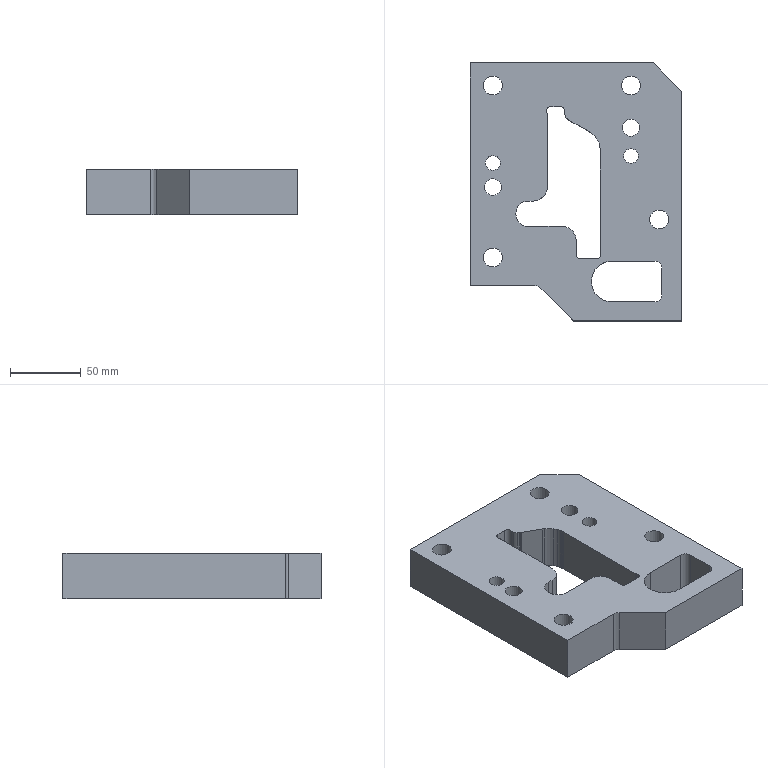Part | STEP file | lll_id130_x_t | 1 solid | 63 faces | box 150 x 183 x 32 mm | volume 623652 mm3 | cylinder 38 | plane 25 | commonest cylinder face diameters 6 x7 13.509 x4 20.008 x4 12 x3 10 x2 10.505 x2